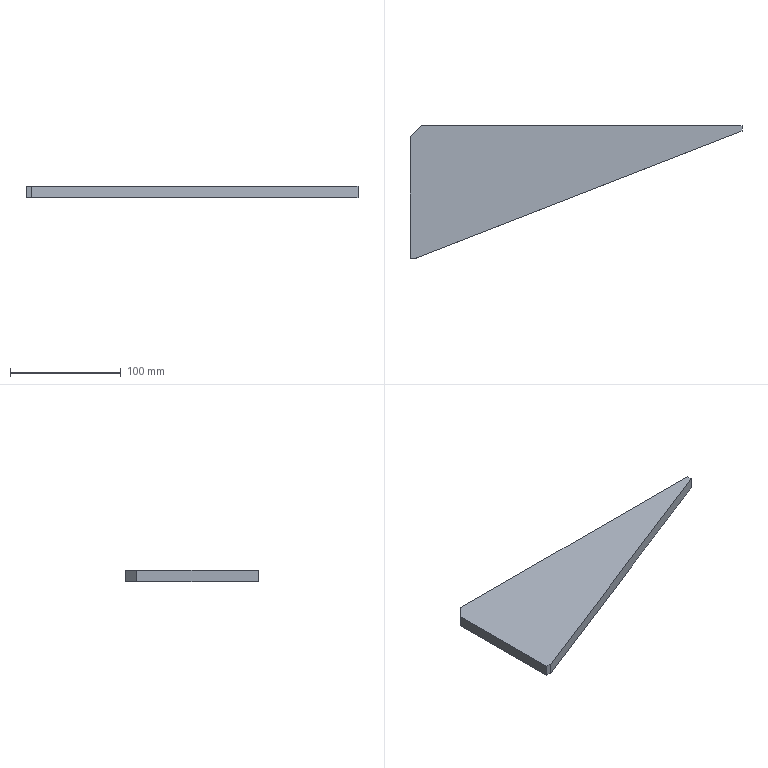Part | STEP file | Positioning_id1582_x_t | 1 solid | 8 faces | box 300 x 120 x 10 mm | volume 189875 mm3 | plane 8
STEP:
#1=CARTESIAN_POINT('',(0.,0.,0.));
#2=DIRECTION('',(0.,0.,1.));
#3=DIRECTION('',(1.,0.,0.));
#4=AXIS2_PLACEMENT_3D('',#1,#2,#3);
#5=CARTESIAN_POINT('',(-1493.002,750.,267.466));
#6=VERTEX_POINT('',#5);
#7=CARTESIAN_POINT('',(-1483.002,760.,267.466));
#8=VERTEX_POINT('',#7);
#9=CARTESIAN_POINT('',(-1493.002,750.,267.466));
#10=DIRECTION('',(0.7071,0.7071,0.));
#11=VECTOR('',#10,1.);
#12=LINE('',#9,#11);
#13=CARTESIAN_POINT('',(-1483.002,760.,262.466));
#14=DIRECTION('',(0.7071,-0.7071,0.));
#15=DIRECTION('',(0.7071,0.7071,0.));
#16=AXIS2_PLACEMENT_3D('',#13,#14,#15);
#17=PLANE('',#16);
#18=CARTESIAN_POINT('',(-14.142,5.));
#19=DIRECTION('',(1.,0.));
#20=VECTOR('',#19,1.);
#21=LINE('',#18,#20);
#22=(GEOMETRIC_REPRESENTATION_CONTEXT(2)PARAMETRIC_REPRESENTATION_CONTEXT()REPRESENTATION_CONTEXT('',''));
#23=DEFINITIONAL_REPRESENTATION('',(#21),#22);
#24=PCURVE('',#17,#23);
#25=CARTESIAN_POINT('',(-1493.002,710.,267.466));
#26=DIRECTION('',(0.,0.,1.));
#27=DIRECTION('',(1.,0.,0.));
#28=AXIS2_PLACEMENT_3D('',#25,#26,#27);
#29=PLANE('',#28);
#30=CARTESIAN_POINT('',(0.,40.));
#31=DIRECTION('',(0.7071,0.7071));
#32=VECTOR('',#31,1.);
#33=LINE('',#30,#32);
#34=(GEOMETRIC_REPRESENTATION_CONTEXT(2)PARAMETRIC_REPRESENTATION_CONTEXT()REPRESENTATION_CONTEXT('',''));
#35=DEFINITIONAL_REPRESENTATION('',(#33),#34);
#36=PCURVE('',#29,#35);
#37=SURFACE_CURVE('',#12,(#24,#36),.PCURVE_S1.);
#38=EDGE_CURVE('',#6,#8,#37,.T.);
#39=ORIENTED_EDGE('',*,*,#38,.T.);
#40=CARTESIAN_POINT('',(-1483.002,760.,257.466));
#41=VERTEX_POINT('',#40);
#42=CARTESIAN_POINT('',(-1483.002,760.,267.466));
#43=DIRECTION('',(0.,0.,-1.));
#44=VECTOR('',#43,1.);
#45=LINE('',#42,#44);
#46=CARTESIAN_POINT('',(0.,5.));
#47=DIRECTION('',(0.,-1.));
#48=VECTOR('',#47,1.);
#49=LINE('',#46,#48);
#50=(GEOMETRIC_REPRESENTATION_CONTEXT(2)PARAMETRIC_REPRESENTATION_CONTEXT()REPRESENTATION_CONTEXT('',''));
#51=DEFINITIONAL_REPRESENTATION('',(#49),#50);
#52=PCURVE('',#17,#51);
#53=CARTESIAN_POINT('',(-1493.002,760.,262.466));
#54=DIRECTION('',(0.,1.,0.));
#55=DIRECTION('',(-1.,0.,0.));
#56=AXIS2_PLACEMENT_3D('',#53,#54,#55);
#57=PLANE('',#56);
#58=CARTESIAN_POINT('',(-10.,5.));
#59=DIRECTION('',(0.,-1.));
#60=VECTOR('',#59,1.);
#61=LINE('',#58,#60);
#62=(GEOMETRIC_REPRESENTATION_CONTEXT(2)PARAMETRIC_REPRESENTATION_CONTEXT()REPRESENTATION_CONTEXT('',''));
#63=DEFINITIONAL_REPRESENTATION('',(#61),#62);
#64=PCURVE('',#57,#63);
#65=SURFACE_CURVE('',#45,(#52,#64),.PCURVE_S1.);
#66=EDGE_CURVE('',#8,#41,#65,.T.);
#67=ORIENTED_EDGE('',*,*,#66,.T.);
#68=CARTESIAN_POINT('',(-1493.002,750.,257.466));
#69=VERTEX_POINT('',#68);
#70=CARTESIAN_POINT('',(-1483.002,760.,257.466));
#71=DIRECTION('',(-0.7071,-0.7071,0.));
#72=VECTOR('',#71,1.);
#73=LINE('',#70,#72);
#74=CARTESIAN_POINT('',(0.,-5.));
#75=DIRECTION('',(-1.,0.));
#76=VECTOR('',#75,1.);
#77=LINE('',#74,#76);
#78=(GEOMETRIC_REPRESENTATION_CONTEXT(2)PARAMETRIC_REPRESENTATION_CONTEXT()REPRESENTATION_CONTEXT('',''));
#79=DEFINITIONAL_REPRESENTATION('',(#77),#78);
#80=PCURVE('',#17,#79);
#81=CARTESIAN_POINT('',(-1493.002,710.,257.466));
#82=DIRECTION('',(0.,0.,-1.));
#83=DIRECTION('',(-1.,0.,0.));
#84=AXIS2_PLACEMENT_3D('',#81,#82,#83);
#85=PLANE('',#84);
#86=CARTESIAN_POINT('',(-10.,50.));
#87=DIRECTION('',(0.7071,-0.7071));
#88=VECTOR('',#87,1.);
#89=LINE('',#86,#88);
#90=(GEOMETRIC_REPRESENTATION_CONTEXT(2)PARAMETRIC_REPRESENTATION_CONTEXT()REPRESENTATION_CONTEXT('',''));
#91=DEFINITIONAL_REPRESENTATION('',(#89),#90);
#92=PCURVE('',#85,#91);
#93=SURFACE_CURVE('',#73,(#80,#92),.PCURVE_S1.);
#94=EDGE_CURVE('',#41,#69,#93,.T.);
#95=ORIENTED_EDGE('',*,*,#94,.T.);
#96=CARTESIAN_POINT('',(-1493.002,750.,257.466));
#97=DIRECTION('',(0.,0.,1.));
#98=VECTOR('',#97,1.);
#99=LINE('',#96,#98);
#100=CARTESIAN_POINT('',(-14.142,-5.));
#101=DIRECTION('',(0.,1.));
#102=VECTOR('',#101,1.);
#103=LINE('',#100,#102);
#104=(GEOMETRIC_REPRESENTATION_CONTEXT(2)PARAMETRIC_REPRESENTATION_CONTEXT()REPRESENTATION_CONTEXT('',''));
#105=DEFINITIONAL_REPRESENTATION('',(#103),#104);
#106=PCURVE('',#17,#105);
#107=CARTESIAN_POINT('',(-1493.002,710.,262.466));
#108=DIRECTION('',(-1.,0.,0.));
#109=DIRECTION('',(0.,0.,1.));
#110=AXIS2_PLACEMENT_3D('',#107,#108,#109);
#111=PLANE('',#110);
#112=CARTESIAN_POINT('',(-5.,40.));
#113=DIRECTION('',(1.,0.));
#114=VECTOR('',#113,1.);
#115=LINE('',#112,#114);
#116=(GEOMETRIC_REPRESENTATION_CONTEXT(2)PARAMETRIC_REPRESENTATION_CONTEXT()REPRESENTATION_CONTEXT('',''));
#117=DEFINITIONAL_REPRESENTATION('',(#115),#116);
#118=PCURVE('',#111,#117);
#119=SURFACE_CURVE('',#99,(#106,#118),.PCURVE_S1.);
#120=EDGE_CURVE('',#69,#6,#119,.T.);
#121=ORIENTED_EDGE('',*,*,#120,.T.);
#122=EDGE_LOOP('',(#39,#67,#95,#121));
#123=FACE_BOUND('',#122,.T.);
#124=ADVANCED_FACE('',(#123),#17,.F.);
#125=CARTESIAN_POINT('',(-1488.002,640.,257.466));
#126=VERTEX_POINT('',#125);
#127=CARTESIAN_POINT('',(-1193.002,755.,257.466));
#128=VERTEX_POINT('',#127);
#129=CARTESIAN_POINT('',(-1488.002,640.,257.466));
#130=DIRECTION('',(0.9317,0.3632,0.));
#131=VECTOR('',#130,1.);
#132=LINE('',#129,#131);
#133=CARTESIAN_POINT('',(-1193.002,755.,262.466));
#134=DIRECTION('',(-0.3632,0.9317,0.));
#135=DIRECTION('',(-0.9317,-0.3632,0.));
#136=AXIS2_PLACEMENT_3D('',#133,#134,#135);
#137=PLANE('',#136);
#138=CARTESIAN_POINT('',(316.623,-5.));
#139=DIRECTION('',(-1.,0.));
#140=VECTOR('',#139,1.);
#141=LINE('',#138,#140);
#142=(GEOMETRIC_REPRESENTATION_CONTEXT(2)PARAMETRIC_REPRESENTATION_CONTEXT()REPRESENTATION_CONTEXT('',''));
#143=DEFINITIONAL_REPRESENTATION('',(#141),#142);
#144=PCURVE('',#137,#143);
#145=CARTESIAN_POINT('',(-5.,-70.));
#146=DIRECTION('',(-0.9317,0.3632));
#147=VECTOR('',#146,1.);
#148=LINE('',#145,#147);
#149=(GEOMETRIC_REPRESENTATION_CONTEXT(2)PARAMETRIC_REPRESENTATION_CONTEXT()REPRESENTATION_CONTEXT('',''));
#150=DEFINITIONAL_REPRESENTATION('',(#148),#149);
#151=PCURVE('',#85,#150);
#152=SURFACE_CURVE('',#132,(#144,#151),.PCURVE_S1.);
#153=EDGE_CURVE('',#126,#128,#152,.T.);
#154=ORIENTED_EDGE('',*,*,#153,.T.);
#155=CARTESIAN_POINT('',(-1193.002,755.,267.466));
#156=VERTEX_POINT('',#155);
#157=CARTESIAN_POINT('',(-1193.002,755.,257.466));
#158=DIRECTION('',(0.,0.,1.));
#159=VECTOR('',#158,1.);
#160=LINE('',#157,#159);
#161=CARTESIAN_POINT('',(0.,-5.));
#162=DIRECTION('',(0.,1.));
#163=VECTOR('',#162,1.);
#164=LINE('',#161,#163);
#165=(GEOMETRIC_REPRESENTATION_CONTEXT(2)PARAMETRIC_REPRESENTATION_CONTEXT()REPRESENTATION_CONTEXT('',''));
#166=DEFINITIONAL_REPRESENTATION('',(#164),#165);
#167=PCURVE('',#137,#166);
#168=CARTESIAN_POINT('',(-1193.002,710.,262.466));
#169=DIRECTION('',(1.,0.,0.));
#170=DIRECTION('',(0.,0.,-1.));
#171=AXIS2_PLACEMENT_3D('',#168,#169,#170);
#172=PLANE('',#171);
#173=CARTESIAN_POINT('',(5.,45.));
#174=DIRECTION('',(-1.,0.));
#175=VECTOR('',#174,1.);
#176=LINE('',#173,#175);
#177=(GEOMETRIC_REPRESENTATION_CONTEXT(2)PARAMETRIC_REPRESENTATION_CONTEXT()REPRESENTATION_CONTEXT('',''));
#178=DEFINITIONAL_REPRESENTATION('',(#176),#177);
#179=PCURVE('',#172,#178);
#180=SURFACE_CURVE('',#160,(#167,#179),.PCURVE_S1.);
#181=EDGE_CURVE('',#128,#156,#180,.T.);
#182=ORIENTED_EDGE('',*,*,#181,.T.);
#183=CARTESIAN_POINT('',(-1488.002,640.,267.466));
#184=VERTEX_POINT('',#183);
#185=CARTESIAN_POINT('',(-1193.002,755.,267.466));
#186=DIRECTION('',(-0.9317,-0.3632,0.));
#187=VECTOR('',#186,1.);
#188=LINE('',#185,#187);
#189=CARTESIAN_POINT('',(0.,5.));
#190=DIRECTION('',(1.,0.));
#191=VECTOR('',#190,1.);
#192=LINE('',#189,#191);
#193=(GEOMETRIC_REPRESENTATION_CONTEXT(2)PARAMETRIC_REPRESENTATION_CONTEXT()REPRESENTATION_CONTEXT('',''));
#194=DEFINITIONAL_REPRESENTATION('',(#192),#193);
#195=PCURVE('',#137,#194);
#196=CARTESIAN_POINT('',(300.,45.));
#197=DIRECTION('',(-0.9317,-0.3632));
#198=VECTOR('',#197,1.);
#199=LINE('',#196,#198);
#200=(GEOMETRIC_REPRESENTATION_CONTEXT(2)PARAMETRIC_REPRESENTATION_CONTEXT()REPRESENTATION_CONTEXT('',''));
#201=DEFINITIONAL_REPRESENTATION('',(#199),#200);
#202=PCURVE('',#29,#201);
#203=SURFACE_CURVE('',#188,(#195,#202),.PCURVE_S1.);
#204=EDGE_CURVE('',#156,#184,#203,.T.);
#205=ORIENTED_EDGE('',*,*,#204,.T.);
#206=CARTESIAN_POINT('',(-1488.002,640.,267.466));
#207=DIRECTION('',(0.,0.,-1.));
#208=VECTOR('',#207,1.);
#209=LINE('',#206,#208);
#210=CARTESIAN_POINT('',(316.623,5.));
#211=DIRECTION('',(0.,-1.));
#212=VECTOR('',#211,1.);
#213=LINE('',#210,#212);
#214=(GEOMETRIC_REPRESENTATION_CONTEXT(2)PARAMETRIC_REPRESENTATION_CONTEXT()REPRESENTATION_CONTEXT('',''));
#215=DEFINITIONAL_REPRESENTATION('',(#213),#214);
#216=PCURVE('',#137,#215);
#217=CARTESIAN_POINT('',(-1493.002,640.,262.466));
#218=DIRECTION('',(0.,-1.,0.));
#219=DIRECTION('',(1.,0.,0.));
#220=AXIS2_PLACEMENT_3D('',#217,#218,#219);
#221=PLANE('',#220);
#222=CARTESIAN_POINT('',(5.,5.));
#223=DIRECTION('',(0.,-1.));
#224=VECTOR('',#223,1.);
#225=LINE('',#222,#224);
#226=(GEOMETRIC_REPRESENTATION_CONTEXT(2)PARAMETRIC_REPRESENTATION_CONTEXT()REPRESENTATION_CONTEXT('',''));
#227=DEFINITIONAL_REPRESENTATION('',(#225),#226);
#228=PCURVE('',#221,#227);
#229=SURFACE_CURVE('',#209,(#216,#228),.PCURVE_S1.);
#230=EDGE_CURVE('',#184,#126,#229,.T.);
#231=ORIENTED_EDGE('',*,*,#230,.T.);
#232=EDGE_LOOP('',(#154,#182,#205,#231));
#233=FACE_BOUND('',#232,.T.);
#234=ADVANCED_FACE('',(#233),#137,.F.);
#235=CARTESIAN_POINT('',(-1493.002,640.,267.466));
#236=VERTEX_POINT('',#235);
#237=CARTESIAN_POINT('',(-1493.002,640.,267.466));
#238=DIRECTION('',(0.,1.,0.));
#239=VECTOR('',#238,1.);
#240=LINE('',#237,#239);
#241=CARTESIAN_POINT('',(0.,-70.));
#242=DIRECTION('',(0.,1.));
#243=VECTOR('',#242,1.);
#244=LINE('',#241,#243);
#245=(GEOMETRIC_REPRESENTATION_CONTEXT(2)PARAMETRIC_REPRESENTATION_CONTEXT()REPRESENTATION_CONTEXT('',''));
#246=DEFINITIONAL_REPRESENTATION('',(#244),#245);
#247=PCURVE('',#29,#246);
#248=CARTESIAN_POINT('',(5.,-70.));
#249=DIRECTION('',(0.,1.));
#250=VECTOR('',#249,1.);
#251=LINE('',#248,#250);
#252=(GEOMETRIC_REPRESENTATION_CONTEXT(2)PARAMETRIC_REPRESENTATION_CONTEXT()REPRESENTATION_CONTEXT('',''));
#253=DEFINITIONAL_REPRESENTATION('',(#251),#252);
#254=PCURVE('',#111,#253);
#255=SURFACE_CURVE('',#240,(#247,#254),.PCURVE_S1.);
#256=EDGE_CURVE('',#236,#6,#255,.T.);
#257=ORIENTED_EDGE('',*,*,#256,.F.);
#258=CARTESIAN_POINT('',(-1493.002,640.,267.466));
#259=DIRECTION('',(1.,0.,0.));
#260=VECTOR('',#259,1.);
#261=LINE('',#258,#260);
#262=CARTESIAN_POINT('',(0.,-70.));
#263=DIRECTION('',(1.,0.));
#264=VECTOR('',#263,1.);
#265=LINE('',#262,#264);
#266=(GEOMETRIC_REPRESENTATION_CONTEXT(2)PARAMETRIC_REPRESENTATION_CONTEXT()REPRESENTATION_CONTEXT('',''));
#267=DEFINITIONAL_REPRESENTATION('',(#265),#266);
#268=PCURVE('',#29,#267);
#269=CARTESIAN_POINT('',(0.,5.));
#270=DIRECTION('',(1.,0.));
#271=VECTOR('',#270,1.);
#272=LINE('',#269,#271);
#273=(GEOMETRIC_REPRESENTATION_CONTEXT(2)PARAMETRIC_REPRESENTATION_CONTEXT()REPRESENTATION_CONTEXT('',''));
#274=DEFINITIONAL_REPRESENTATION('',(#272),#273);
#275=PCURVE('',#221,#274);
#276=SURFACE_CURVE('',#261,(#268,#275),.PCURVE_S1.);
#277=EDGE_CURVE('',#236,#184,#276,.T.);
#278=ORIENTED_EDGE('',*,*,#277,.T.);
#279=ORIENTED_EDGE('',*,*,#204,.F.);
#280=CARTESIAN_POINT('',(-1193.002,760.,267.466));
#281=VERTEX_POINT('',#280);
#282=CARTESIAN_POINT('',(-1193.002,760.,267.466));
#283=DIRECTION('',(0.,-1.,0.));
#284=VECTOR('',#283,1.);
#285=LINE('',#282,#284);
#286=CARTESIAN_POINT('',(300.,50.));
#287=DIRECTION('',(0.,-1.));
#288=VECTOR('',#287,1.);
#289=LINE('',#286,#288);
#290=(GEOMETRIC_REPRESENTATION_CONTEXT(2)PARAMETRIC_REPRESENTATION_CONTEXT()REPRESENTATION_CONTEXT('',''));
#291=DEFINITIONAL_REPRESENTATION('',(#289),#290);
#292=PCURVE('',#29,#291);
#293=CARTESIAN_POINT('',(-5.,50.));
#294=DIRECTION('',(0.,-1.));
#295=VECTOR('',#294,1.);
#296=LINE('',#293,#295);
#297=(GEOMETRIC_REPRESENTATION_CONTEXT(2)PARAMETRIC_REPRESENTATION_CONTEXT()REPRESENTATION_CONTEXT('',''));
#298=DEFINITIONAL_REPRESENTATION('',(#296),#297);
#299=PCURVE('',#172,#298);
#300=SURFACE_CURVE('',#285,(#292,#299),.PCURVE_S1.);
#301=EDGE_CURVE('',#281,#156,#300,.T.);
#302=ORIENTED_EDGE('',*,*,#301,.F.);
#303=CARTESIAN_POINT('',(-1483.002,760.,267.466));
#304=DIRECTION('',(1.,0.,0.));
#305=VECTOR('',#304,1.);
#306=LINE('',#303,#305);
#307=CARTESIAN_POINT('',(10.,50.));
#308=DIRECTION('',(1.,0.));
#309=VECTOR('',#308,1.);
#310=LINE('',#307,#309);
#311=(GEOMETRIC_REPRESENTATION_CONTEXT(2)PARAMETRIC_REPRESENTATION_CONTEXT()REPRESENTATION_CONTEXT('',''));
#312=DEFINITIONAL_REPRESENTATION('',(#310),#311);
#313=PCURVE('',#29,#312);
#314=CARTESIAN_POINT('',(-10.,5.));
#315=DIRECTION('',(-1.,0.));
#316=VECTOR('',#315,1.);
#317=LINE('',#314,#316);
#318=(GEOMETRIC_REPRESENTATION_CONTEXT(2)PARAMETRIC_REPRESENTATION_CONTEXT()REPRESENTATION_CONTEXT('',''));
#319=DEFINITIONAL_REPRESENTATION('',(#317),#318);
#320=PCURVE('',#57,#319);
#321=SURFACE_CURVE('',#306,(#313,#320),.PCURVE_S1.);
#322=EDGE_CURVE('',#8,#281,#321,.T.);
#323=ORIENTED_EDGE('',*,*,#322,.F.);
#324=ORIENTED_EDGE('',*,*,#38,.F.);
#325=EDGE_LOOP('',(#257,#278,#279,#302,#323,#324));
#326=FACE_BOUND('',#325,.T.);
#327=ADVANCED_FACE('',(#326),#29,.T.);
#328=CARTESIAN_POINT('',(-1493.002,640.,257.466));
#329=VERTEX_POINT('',#328);
#330=CARTESIAN_POINT('',(-1493.002,750.,257.466));
#331=DIRECTION('',(0.,-1.,0.));
#332=VECTOR('',#331,1.);
#333=LINE('',#330,#332);
#334=CARTESIAN_POINT('',(-5.,40.));
#335=DIRECTION('',(0.,-1.));
#336=VECTOR('',#335,1.);
#337=LINE('',#334,#336);
#338=(GEOMETRIC_REPRESENTATION_CONTEXT(2)PARAMETRIC_REPRESENTATION_CONTEXT()REPRESENTATION_CONTEXT('',''));
#339=DEFINITIONAL_REPRESENTATION('',(#337),#338);
#340=PCURVE('',#111,#339);
#341=CARTESIAN_POINT('',(0.,40.));
#342=DIRECTION('',(0.,-1.));
#343=VECTOR('',#342,1.);
#344=LINE('',#341,#343);
#345=(GEOMETRIC_REPRESENTATION_CONTEXT(2)PARAMETRIC_REPRESENTATION_CONTEXT()REPRESENTATION_CONTEXT('',''));
#346=DEFINITIONAL_REPRESENTATION('',(#344),#345);
#347=PCURVE('',#85,#346);
#348=SURFACE_CURVE('',#333,(#340,#347),.PCURVE_S1.);
#349=EDGE_CURVE('',#69,#329,#348,.T.);
#350=ORIENTED_EDGE('',*,*,#349,.T.);
#351=CARTESIAN_POINT('',(-1493.002,640.,257.466));
#352=DIRECTION('',(0.,0.,1.));
#353=VECTOR('',#352,1.);
#354=LINE('',#351,#353);
#355=CARTESIAN_POINT('',(-5.,-70.));
#356=DIRECTION('',(1.,0.));
#357=VECTOR('',#356,1.);
#358=LINE('',#355,#357);
#359=(GEOMETRIC_REPRESENTATION_CONTEXT(2)PARAMETRIC_REPRESENTATION_CONTEXT()REPRESENTATION_CONTEXT('',''));
#360=DEFINITIONAL_REPRESENTATION('',(#358),#359);
#361=PCURVE('',#111,#360);
#362=CARTESIAN_POINT('',(0.,-5.));
#363=DIRECTION('',(0.,1.));
#364=VECTOR('',#363,1.);
#365=LINE('',#362,#364);
#366=(GEOMETRIC_REPRESENTATION_CONTEXT(2)PARAMETRIC_REPRESENTATION_CONTEXT()REPRESENTATION_CONTEXT('',''));
#367=DEFINITIONAL_REPRESENTATION('',(#365),#366);
#368=PCURVE('',#221,#367);
#369=SURFACE_CURVE('',#354,(#361,#368),.PCURVE_S1.);
#370=EDGE_CURVE('',#329,#236,#369,.T.);
#371=ORIENTED_EDGE('',*,*,#370,.T.);
#372=ORIENTED_EDGE('',*,*,#256,.T.);
#373=ORIENTED_EDGE('',*,*,#120,.F.);
#374=EDGE_LOOP('',(#350,#371,#372,#373));
#375=FACE_BOUND('',#374,.T.);
#376=ADVANCED_FACE('',(#375),#111,.T.);
#377=ORIENTED_EDGE('',*,*,#322,.T.);
#378=CARTESIAN_POINT('',(-1193.002,760.,257.466));
#379=VERTEX_POINT('',#378);
#380=CARTESIAN_POINT('',(-1193.002,760.,257.466));
#381=DIRECTION('',(0.,0.,1.));
#382=VECTOR('',#381,1.);
#383=LINE('',#380,#382);
#384=CARTESIAN_POINT('',(-300.,-5.));
#385=DIRECTION('',(0.,1.));
#386=VECTOR('',#385,1.);
#387=LINE('',#384,#386);
#388=(GEOMETRIC_REPRESENTATION_CONTEXT(2)PARAMETRIC_REPRESENTATION_CONTEXT()REPRESENTATION_CONTEXT('',''));
#389=DEFINITIONAL_REPRESENTATION('',(#387),#388);
#390=PCURVE('',#57,#389);
#391=CARTESIAN_POINT('',(5.,50.));
#392=DIRECTION('',(-1.,0.));
#393=VECTOR('',#392,1.);
#394=LINE('',#391,#393);
#395=(GEOMETRIC_REPRESENTATION_CONTEXT(2)PARAMETRIC_REPRESENTATION_CONTEXT()REPRESENTATION_CONTEXT('',''));
#396=DEFINITIONAL_REPRESENTATION('',(#394),#395);
#397=PCURVE('',#172,#396);
#398=SURFACE_CURVE('',#383,(#390,#397),.PCURVE_S1.);
#399=EDGE_CURVE('',#379,#281,#398,.T.);
#400=ORIENTED_EDGE('',*,*,#399,.F.);
#401=CARTESIAN_POINT('',(-1483.002,760.,257.466));
#402=DIRECTION('',(1.,0.,0.));
#403=VECTOR('',#402,1.);
#404=LINE('',#401,#403);
#405=CARTESIAN_POINT('',(-10.,-5.));
#406=DIRECTION('',(-1.,0.));
#407=VECTOR('',#406,1.);
#408=LINE('',#405,#407);
#409=(GEOMETRIC_REPRESENTATION_CONTEXT(2)PARAMETRIC_REPRESENTATION_CONTEXT()REPRESENTATION_CONTEXT('',''));
#410=DEFINITIONAL_REPRESENTATION('',(#408),#409);
#411=PCURVE('',#57,#410);
#412=CARTESIAN_POINT('',(-10.,50.));
#413=DIRECTION('',(-1.,0.));
#414=VECTOR('',#413,1.);
#415=LINE('',#412,#414);
#416=(GEOMETRIC_REPRESENTATION_CONTEXT(2)PARAMETRIC_REPRESENTATION_CONTEXT()REPRESENTATION_CONTEXT('',''));
#417=DEFINITIONAL_REPRESENTATION('',(#415),#416);
#418=PCURVE('',#85,#417);
#419=SURFACE_CURVE('',#404,(#411,#418),.PCURVE_S1.);
#420=EDGE_CURVE('',#41,#379,#419,.T.);
#421=ORIENTED_EDGE('',*,*,#420,.F.);
#422=ORIENTED_EDGE('',*,*,#66,.F.);
#423=EDGE_LOOP('',(#377,#400,#421,#422));
#424=FACE_BOUND('',#423,.T.);
#425=ADVANCED_FACE('',(#424),#57,.T.);
#426=ORIENTED_EDGE('',*,*,#420,.T.);
#427=CARTESIAN_POINT('',(-1193.002,755.,257.466));
#428=DIRECTION('',(0.,1.,0.));
#429=VECTOR('',#428,1.);
#430=LINE('',#427,#429);
#431=CARTESIAN_POINT('',(-300.,45.));
#432=DIRECTION('',(0.,1.));
#433=VECTOR('',#432,1.);
#434=LINE('',#431,#433);
#435=(GEOMETRIC_REPRESENTATION_CONTEXT(2)PARAMETRIC_REPRESENTATION_CONTEXT()REPRESENTATION_CONTEXT('',''));
#436=DEFINITIONAL_REPRESENTATION('',(#434),#435);
#437=PCURVE('',#85,#436);
#438=CARTESIAN_POINT('',(5.,45.));
#439=DIRECTION('',(0.,1.));
#440=VECTOR('',#439,1.);
#441=LINE('',#438,#440);
#442=(GEOMETRIC_REPRESENTATION_CONTEXT(2)PARAMETRIC_REPRESENTATION_CONTEXT()REPRESENTATION_CONTEXT('',''));
#443=DEFINITIONAL_REPRESENTATION('',(#441),#442);
#444=PCURVE('',#172,#443);
#445=SURFACE_CURVE('',#430,(#437,#444),.PCURVE_S1.);
#446=EDGE_CURVE('',#128,#379,#445,.T.);
#447=ORIENTED_EDGE('',*,*,#446,.F.);
#448=ORIENTED_EDGE('',*,*,#153,.F.);
#449=CARTESIAN_POINT('',(-1493.002,640.,257.466));
#450=DIRECTION('',(1.,0.,0.));
#451=VECTOR('',#450,1.);
#452=LINE('',#449,#451);
#453=CARTESIAN_POINT('',(0.,-70.));
#454=DIRECTION('',(-1.,0.));
#455=VECTOR('',#454,1.);
#456=LINE('',#453,#455);
#457=(GEOMETRIC_REPRESENTATION_CONTEXT(2)PARAMETRIC_REPRESENTATION_CONTEXT()REPRESENTATION_CONTEXT('',''));
#458=DEFINITIONAL_REPRESENTATION('',(#456),#457);
#459=PCURVE('',#85,#458);
#460=CARTESIAN_POINT('',(0.,-5.));
#461=DIRECTION('',(1.,0.));
#462=VECTOR('',#461,1.);
#463=LINE('',#460,#462);
#464=(GEOMETRIC_REPRESENTATION_CONTEXT(2)PARAMETRIC_REPRESENTATION_CONTEXT()REPRESENTATION_CONTEXT('',''));
#465=DEFINITIONAL_REPRESENTATION('',(#463),#464);
#466=PCURVE('',#221,#465);
#467=SURFACE_CURVE('',#452,(#459,#466),.PCURVE_S1.);
#468=EDGE_CURVE('',#329,#126,#467,.T.);
#469=ORIENTED_EDGE('',*,*,#468,.F.);
#470=ORIENTED_EDGE('',*,*,#349,.F.);
#471=ORIENTED_EDGE('',*,*,#94,.F.);
#472=EDGE_LOOP('',(#426,#447,#448,#469,#470,#471));
#473=FACE_BOUND('',#472,.T.);
#474=ADVANCED_FACE('',(#473),#85,.T.);
#475=ORIENTED_EDGE('',*,*,#277,.F.);
#476=ORIENTED_EDGE('',*,*,#370,.F.);
#477=ORIENTED_EDGE('',*,*,#468,.T.);
#478=ORIENTED_EDGE('',*,*,#230,.F.);
#479=EDGE_LOOP('',(#475,#476,#477,#478));
#480=FACE_BOUND('',#479,.T.);
#481=ADVANCED_FACE('',(#480),#221,.T.);
#482=ORIENTED_EDGE('',*,*,#446,.T.);
#483=ORIENTED_EDGE('',*,*,#399,.T.);
#484=ORIENTED_EDGE('',*,*,#301,.T.);
#485=ORIENTED_EDGE('',*,*,#181,.F.);
#486=EDGE_LOOP('',(#482,#483,#484,#485));
#487=FACE_BOUND('',#486,.T.);
#488=ADVANCED_FACE('',(#487),#172,.T.);
#489=CLOSED_SHELL('',(#124,#234,#327,#376,#425,#474,#481,#488));
#490=MANIFOLD_SOLID_BREP('',#489);
#491=(LENGTH_UNIT()NAMED_UNIT(*)SI_UNIT(.MILLI.,.METRE.));
#492=UNCERTAINTY_MEASURE_WITH_UNIT(LENGTH_MEASURE(0.0000001),#491,'','');
#493=(NAMED_UNIT(*)PLANE_ANGLE_UNIT()SI_UNIT($,.RADIAN.));
#494=(NAMED_UNIT(*)SI_UNIT($,.STERADIAN.)SOLID_ANGLE_UNIT());
#495=(GEOMETRIC_REPRESENTATION_CONTEXT(3)GLOBAL_UNCERTAINTY_ASSIGNED_CONTEXT((#492))GLOBAL_UNIT_ASSIGNED_CONTEXT((#491,#493,#494))REPRESENTATION_CONTEXT('',''));
#496=ADVANCED_BREP_SHAPE_REPRESENTATION('',(#4,#490),#495);